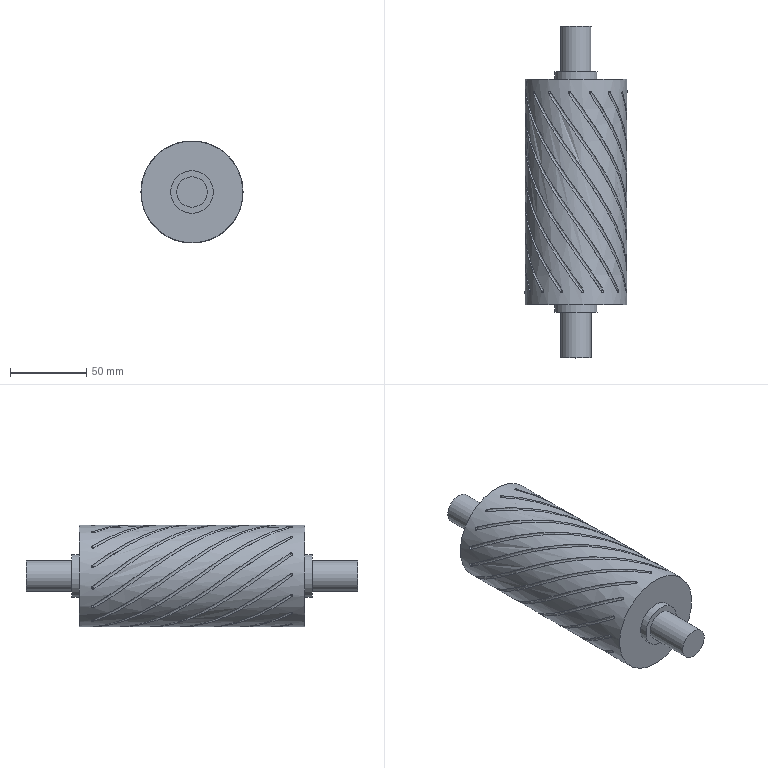Part | STEP file | YBQDJ-YB-5 | 1 solid | 86 faces | box 68.992 x 218 x 68.953 mm | volume 543044 mm3 | spline 45 | plane 36 | cylinder 5 | commonest cylinder face diameters 20 x2 28 x2 67 x1